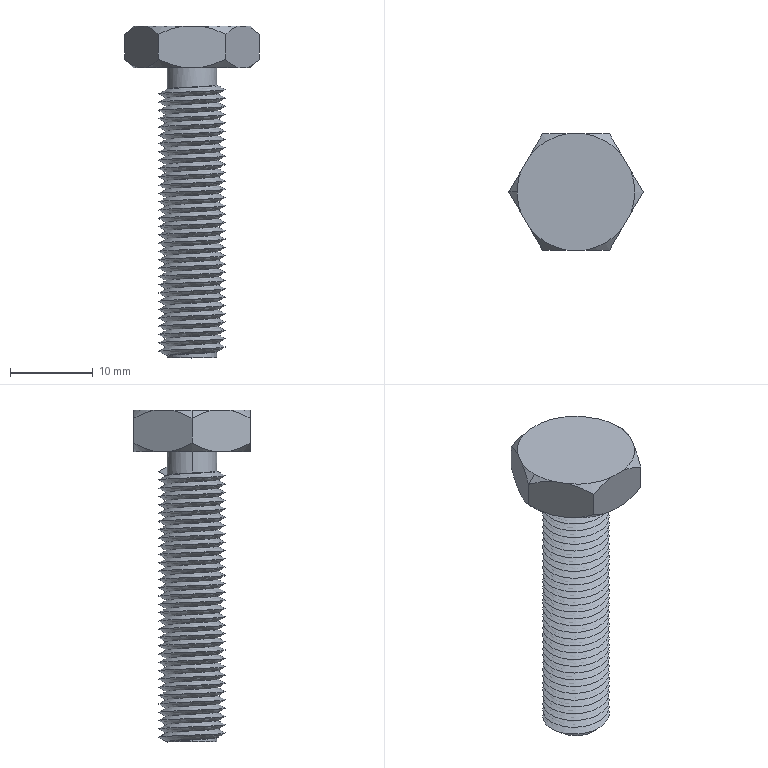Part | SolidWorks | features BaseBody 1 | 1 solid | 34 faces | box 16.166 x 14 x 40 mm | volume 2199 mm3 | cone 14 | plane 11 | cylinder 5 | spline 4 | commonest cylinder face diameters 6 x5